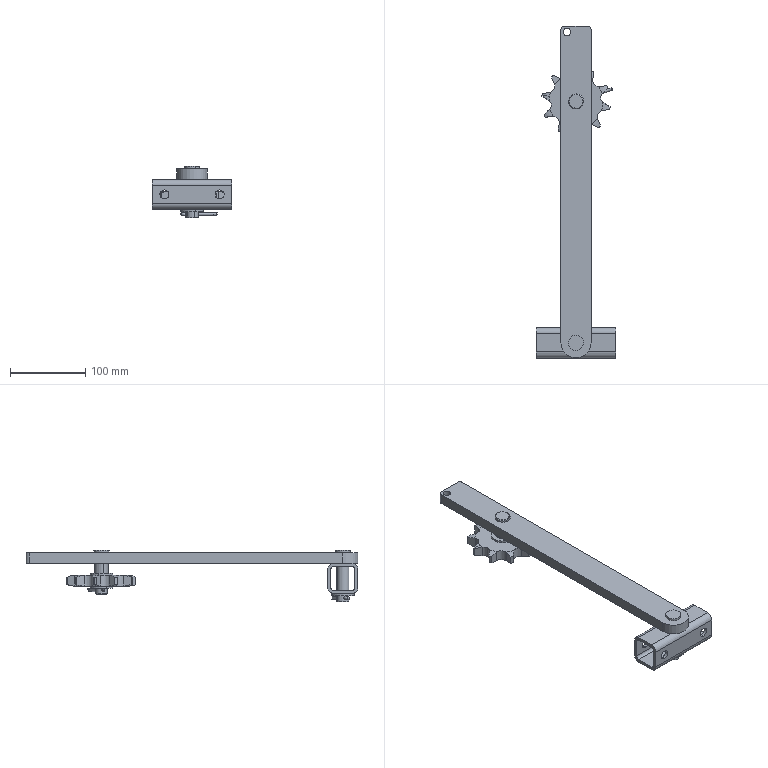Part | SolidWorks | features CompositeCurve 20 | 10 solids | 192 faces | box 105 x 440 x 68.5 mm | volume 381290 mm3 | cylinder 92 | plane 62 | torus 34 | cone 4 | commonest cylinder face diameters 15.88 x14 17 x12 91.8 x11 12 x8 16 x8 30 x6